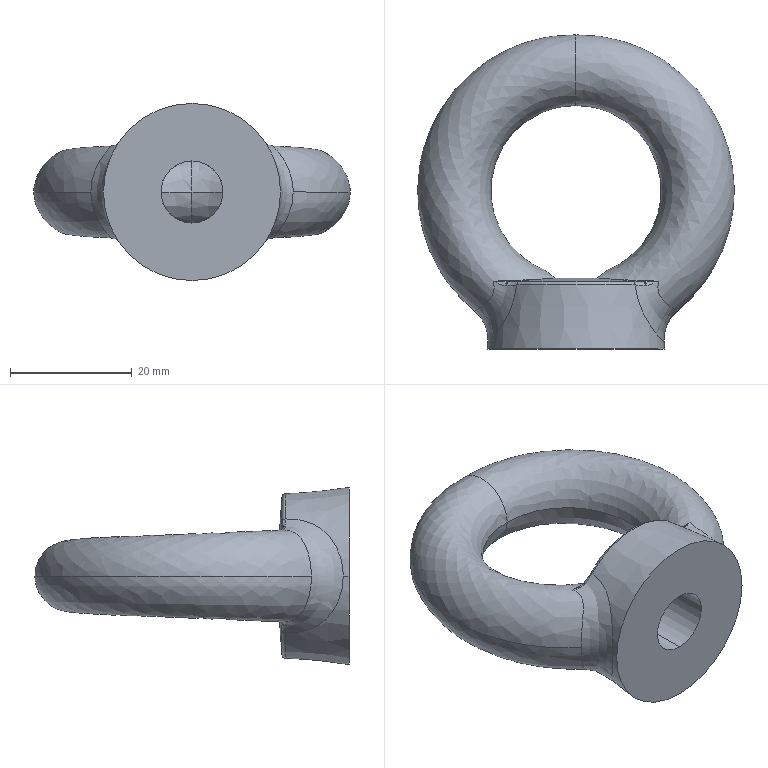Part | STEP file | GB╱T 825-1988[吊环Nut M12] | 1 solid | 27 faces | box 52.011 x 51.603 x 29.1 mm | volume 18454 mm3 | spline 18 | cone 4 | cylinder 2 | torus 2 | plane 1 | commonest cylinder face diameters 10.2 x2